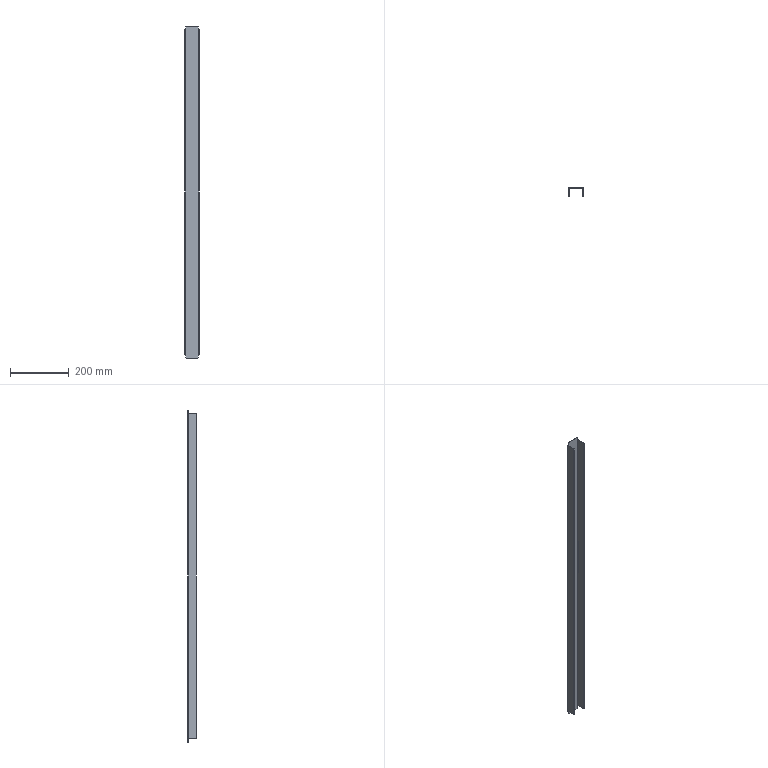Part | SolidWorks | features Chamfer 1, FlatPattern 1, ICE 1, SMBaseFlange 1, SheetMetal 1 | 1 solid | 26 faces | box 50 x 30 x 1127 mm | volume 233640 mm3 | plane 22 | cylinder 4 | commonest cylinder face diameters 0.4 x2 4.4 x2
STEP:
#1=CARTESIAN_POINT('',(-19.,-2.,563.5));
#2=VERTEX_POINT('',#1);
#3=CARTESIAN_POINT('',(19.,-2.,563.5));
#4=VERTEX_POINT('',#3);
#5=CARTESIAN_POINT('',(-25.,-2.,563.5));
#6=DIRECTION('',(1.,0.,0.));
#7=VECTOR('',#6,1000.);
#8=LINE('',#5,#7);
#9=EDGE_CURVE('',#2,#4,#8,.T.);
#10=ORIENTED_EDGE('',*,*,#9,.T.);
#11=CARTESIAN_POINT('',(19.,0.,563.5));
#12=VERTEX_POINT('',#11);
#13=CARTESIAN_POINT('',(19.,0.,563.5));
#14=DIRECTION('',(0.,1.,0.));
#15=VECTOR('',#14,1000.);
#16=LINE('',#13,#15);
#17=EDGE_CURVE('',#4,#12,#16,.T.);
#18=ORIENTED_EDGE('',*,*,#17,.T.);
#19=CARTESIAN_POINT('',(-19.,0.,563.5));
#20=VERTEX_POINT('',#19);
#21=CARTESIAN_POINT('',(-25.,0.,563.5));
#22=DIRECTION('',(1.,0.,0.));
#23=VECTOR('',#22,1000.);
#24=LINE('',#21,#23);
#25=EDGE_CURVE('',#20,#12,#24,.T.);
#26=ORIENTED_EDGE('',*,*,#25,.F.);
#27=CARTESIAN_POINT('',(-19.,-2.,563.5));
#28=DIRECTION('',(0.,-1.,0.));
#29=VECTOR('',#28,1000.);
#30=LINE('',#27,#29);
#31=EDGE_CURVE('',#20,#2,#30,.T.);
#32=ORIENTED_EDGE('',*,*,#31,.T.);
#33=EDGE_LOOP('',(#10,#18,#26,#32));
#34=FACE_OUTER_BOUND('',#33,.T.);
#35=CARTESIAN_POINT('',(-23.,-2.2,563.5));
#36=DIRECTION('',(0.,0.,1.));
#37=DIRECTION('',(1.,0.,0.));
#38=AXIS2_PLACEMENT_3D('',#35,#36,#37);
#39=PLANE('',#38);
#40=ADVANCED_FACE('',(#34),#39,.T.);
#41=CARTESIAN_POINT('',(-19.,0.,-563.5));
#42=VERTEX_POINT('',#41);
#43=CARTESIAN_POINT('',(19.,0.,-563.5));
#44=VERTEX_POINT('',#43);
#45=CARTESIAN_POINT('',(-25.,0.,-563.5));
#46=DIRECTION('',(1.,0.,0.));
#47=VECTOR('',#46,1000.);
#48=LINE('',#45,#47);
#49=EDGE_CURVE('',#42,#44,#48,.T.);
#50=ORIENTED_EDGE('',*,*,#49,.T.);
#51=CARTESIAN_POINT('',(19.,-2.,-563.5));
#52=VERTEX_POINT('',#51);
#53=CARTESIAN_POINT('',(19.,-2.,-563.5));
#54=DIRECTION('',(0.,-1.,0.));
#55=VECTOR('',#54,1000.);
#56=LINE('',#53,#55);
#57=EDGE_CURVE('',#44,#52,#56,.T.);
#58=ORIENTED_EDGE('',*,*,#57,.T.);
#59=CARTESIAN_POINT('',(-19.,-2.,-563.5));
#60=VERTEX_POINT('',#59);
#61=CARTESIAN_POINT('',(-25.,-2.,-563.5));
#62=DIRECTION('',(1.,0.,0.));
#63=VECTOR('',#62,1000.);
#64=LINE('',#61,#63);
#65=EDGE_CURVE('',#60,#52,#64,.T.);
#66=ORIENTED_EDGE('',*,*,#65,.F.);
#67=CARTESIAN_POINT('',(-19.,0.,-563.5));
#68=DIRECTION('',(0.,1.,0.));
#69=VECTOR('',#68,1000.);
#70=LINE('',#67,#69);
#71=EDGE_CURVE('',#60,#42,#70,.T.);
#72=ORIENTED_EDGE('',*,*,#71,.T.);
#73=EDGE_LOOP('',(#50,#58,#66,#72));
#74=FACE_OUTER_BOUND('',#73,.T.);
#75=CARTESIAN_POINT('',(23.,-2.2,-563.5));
#76=DIRECTION('',(0.,0.,-1.));
#77=DIRECTION('',(-1.,0.,0.));
#78=AXIS2_PLACEMENT_3D('',#75,#76,#77);
#79=PLANE('',#78);
#80=ADVANCED_FACE('',(#74),#79,.T.);
#81=CARTESIAN_POINT('',(23.,-2.2,551.5));
#82=VERTEX_POINT('',#81);
#83=CARTESIAN_POINT('',(23.,-2.2,-551.5));
#84=VERTEX_POINT('',#83);
#85=CARTESIAN_POINT('',(23.,-2.2,563.5));
#86=DIRECTION('',(0.,0.,-1.));
#87=VECTOR('',#86,1000.);
#88=LINE('',#85,#87);
#89=EDGE_CURVE('',#82,#84,#88,.T.);
#90=ORIENTED_EDGE('',*,*,#89,.T.);
#91=CARTESIAN_POINT('',(23.,-30.,-551.5));
#92=VERTEX_POINT('',#91);
#93=CARTESIAN_POINT('',(23.,0.,-551.5));
#94=DIRECTION('',(0.,-1.,0.));
#95=VECTOR('',#94,1000.);
#96=LINE('',#93,#95);
#97=EDGE_CURVE('',#84,#92,#96,.T.);
#98=ORIENTED_EDGE('',*,*,#97,.T.);
#99=CARTESIAN_POINT('',(23.,-30.,551.5));
#100=VERTEX_POINT('',#99);
#101=CARTESIAN_POINT('',(23.,-30.,563.5));
#102=DIRECTION('',(0.,0.,-1.));
#103=VECTOR('',#102,1000.);
#104=LINE('',#101,#103);
#105=EDGE_CURVE('',#100,#92,#104,.T.);
#106=ORIENTED_EDGE('',*,*,#105,.F.);
#107=CARTESIAN_POINT('',(23.,0.,551.5));
#108=DIRECTION('',(0.,1.,0.));
#109=VECTOR('',#108,1000.);
#110=LINE('',#107,#109);
#111=EDGE_CURVE('',#100,#82,#110,.T.);
#112=ORIENTED_EDGE('',*,*,#111,.T.);
#113=EDGE_LOOP('',(#90,#98,#106,#112));
#114=FACE_OUTER_BOUND('',#113,.T.);
#115=CARTESIAN_POINT('',(23.,0.,563.5));
#116=DIRECTION('',(1.,0.,0.));
#117=DIRECTION('',(0.,1.,0.));
#118=AXIS2_PLACEMENT_3D('',#115,#116,#117);
#119=PLANE('',#118);
#120=ADVANCED_FACE('',(#114),#119,.F.);
#121=CARTESIAN_POINT('',(25.,-30.,-551.5));
#122=VERTEX_POINT('',#121);
#123=CARTESIAN_POINT('',(25.,-30.,-551.5));
#124=DIRECTION('',(1.,0.,0.));
#125=VECTOR('',#124,1000.);
#126=LINE('',#123,#125);
#127=EDGE_CURVE('',#92,#122,#126,.T.);
#128=ORIENTED_EDGE('',*,*,#127,.T.);
#129=CARTESIAN_POINT('',(25.,-30.,551.5));
#130=VERTEX_POINT('',#129);
#131=CARTESIAN_POINT('',(25.,-30.,563.5));
#132=DIRECTION('',(0.,0.,-1.));
#133=VECTOR('',#132,1000.);
#134=LINE('',#131,#133);
#135=EDGE_CURVE('',#130,#122,#134,.T.);
#136=ORIENTED_EDGE('',*,*,#135,.F.);
#137=CARTESIAN_POINT('',(25.,-30.,551.5));
#138=DIRECTION('',(-1.,0.,0.));
#139=VECTOR('',#138,1000.);
#140=LINE('',#137,#139);
#141=EDGE_CURVE('',#130,#100,#140,.T.);
#142=ORIENTED_EDGE('',*,*,#141,.T.);
#143=ORIENTED_EDGE('',*,*,#105,.T.);
#144=EDGE_LOOP('',(#128,#136,#142,#143));
#145=FACE_OUTER_BOUND('',#144,.T.);
#146=CARTESIAN_POINT('',(25.,-30.,563.5));
#147=DIRECTION('',(0.,-1.,0.));
#148=DIRECTION('',(1.,0.,0.));
#149=AXIS2_PLACEMENT_3D('',#146,#147,#148);
#150=PLANE('',#149);
#151=ADVANCED_FACE('',(#145),#150,.T.);
#152=CARTESIAN_POINT('',(25.,-2.2,-551.5));
#153=VERTEX_POINT('',#152);
#154=CARTESIAN_POINT('',(25.,-30.,-551.5));
#155=DIRECTION('',(0.,1.,0.));
#156=VECTOR('',#155,1000.);
#157=LINE('',#154,#156);
#158=EDGE_CURVE('',#122,#153,#157,.T.);
#159=ORIENTED_EDGE('',*,*,#158,.T.);
#160=CARTESIAN_POINT('',(25.,-2.2,551.5));
#161=VERTEX_POINT('',#160);
#162=CARTESIAN_POINT('',(25.,-2.2,563.5));
#163=DIRECTION('',(0.,0.,-1.));
#164=VECTOR('',#163,1000.);
#165=LINE('',#162,#164);
#166=EDGE_CURVE('',#161,#153,#165,.T.);
#167=ORIENTED_EDGE('',*,*,#166,.F.);
#168=CARTESIAN_POINT('',(25.,-30.,551.5));
#169=DIRECTION('',(0.,1.,0.));
#170=VECTOR('',#169,1000.);
#171=LINE('',#168,#170);
#172=EDGE_CURVE('',#130,#161,#171,.T.);
#173=ORIENTED_EDGE('',*,*,#172,.F.);
#174=ORIENTED_EDGE('',*,*,#135,.T.);
#175=EDGE_LOOP('',(#159,#167,#173,#174));
#176=FACE_OUTER_BOUND('',#175,.T.);
#177=CARTESIAN_POINT('',(25.,0.,563.5));
#178=DIRECTION('',(1.,0.,0.));
#179=DIRECTION('',(0.,1.,0.));
#180=AXIS2_PLACEMENT_3D('',#177,#178,#179);
#181=PLANE('',#180);
#182=ADVANCED_FACE('',(#176),#181,.T.);
#183=CARTESIAN_POINT('',(22.8,0.,-551.5));
#184=VERTEX_POINT('',#183);
#185=CARTESIAN_POINT('',(22.8,-2.2,-551.5));
#186=DIRECTION('',(0.,0.,-1.));
#187=DIRECTION('',(1.,0.,0.));
#188=AXIS2_PLACEMENT_3D('',#185,#186,#187);
#189=CIRCLE('',#188,2.2);
#190=EDGE_CURVE('',#184,#153,#189,.T.);
#191=ORIENTED_EDGE('',*,*,#190,.F.);
#192=CARTESIAN_POINT('',(22.8,0.,551.5));
#193=VERTEX_POINT('',#192);
#194=CARTESIAN_POINT('',(22.8,0.,563.5));
#195=DIRECTION('',(0.,0.,-1.));
#196=VECTOR('',#195,1000.);
#197=LINE('',#194,#196);
#198=EDGE_CURVE('',#193,#184,#197,.T.);
#199=ORIENTED_EDGE('',*,*,#198,.F.);
#200=CARTESIAN_POINT('',(22.8,-2.2,551.5));
#201=DIRECTION('',(0.,0.,1.));
#202=DIRECTION('',(-1.,0.,0.));
#203=AXIS2_PLACEMENT_3D('',#200,#201,#202);
#204=CIRCLE('',#203,2.2);
#205=EDGE_CURVE('',#161,#193,#204,.T.);
#206=ORIENTED_EDGE('',*,*,#205,.F.);
#207=ORIENTED_EDGE('',*,*,#166,.T.);
#208=EDGE_LOOP('',(#191,#199,#206,#207));
#209=FACE_OUTER_BOUND('',#208,.T.);
#210=CARTESIAN_POINT('',(22.8,-2.2,563.5));
#211=DIRECTION('',(0.,0.,-1.));
#212=DIRECTION('',(-1.,0.,0.));
#213=AXIS2_PLACEMENT_3D('',#210,#211,#212);
#214=CYLINDRICAL_SURFACE('',#213,2.2);
#215=ADVANCED_FACE('',(#209),#214,.T.);
#216=CARTESIAN_POINT('',(22.,0.,-560.5));
#217=VERTEX_POINT('',#216);
#218=CARTESIAN_POINT('',(22.,0.,-551.5));
#219=VERTEX_POINT('',#218);
#220=CARTESIAN_POINT('',(22.,0.,563.5));
#221=DIRECTION('',(0.,0.,1.));
#222=VECTOR('',#221,1000.);
#223=LINE('',#220,#222);
#224=EDGE_CURVE('',#217,#219,#223,.T.);
#225=ORIENTED_EDGE('',*,*,#224,.F.);
#226=CARTESIAN_POINT('',(560.5,0.,-22.));
#227=DIRECTION('',(-0.7071,0.,-0.7071));
#228=VECTOR('',#227,1000.);
#229=LINE('',#226,#228);
#230=EDGE_CURVE('',#217,#44,#229,.T.);
#231=ORIENTED_EDGE('',*,*,#230,.T.);
#232=ORIENTED_EDGE('',*,*,#49,.F.);
#233=CARTESIAN_POINT('',(-22.,0.,-560.5));
#234=VERTEX_POINT('',#233);
#235=CARTESIAN_POINT('',(-585.5,0.,3.));
#236=DIRECTION('',(-0.7071,0.,0.7071));
#237=VECTOR('',#236,1000.);
#238=LINE('',#235,#237);
#239=EDGE_CURVE('',#42,#234,#238,.T.);
#240=ORIENTED_EDGE('',*,*,#239,.T.);
#241=CARTESIAN_POINT('',(-22.,0.,-551.5));
#242=VERTEX_POINT('',#241);
#243=CARTESIAN_POINT('',(-22.,0.,563.5));
#244=DIRECTION('',(0.,0.,-1.));
#245=VECTOR('',#244,1000.);
#246=LINE('',#243,#245);
#247=EDGE_CURVE('',#242,#234,#246,.T.);
#248=ORIENTED_EDGE('',*,*,#247,.F.);
#249=CARTESIAN_POINT('',(-22.8,0.,-551.5));
#250=VERTEX_POINT('',#249);
#251=CARTESIAN_POINT('',(-25.,0.,-551.5));
#252=DIRECTION('',(1.,0.,0.));
#253=VECTOR('',#252,1000.);
#254=LINE('',#251,#253);
#255=EDGE_CURVE('',#250,#242,#254,.T.);
#256=ORIENTED_EDGE('',*,*,#255,.F.);
#257=CARTESIAN_POINT('',(-22.8,0.,551.5));
#258=VERTEX_POINT('',#257);
#259=CARTESIAN_POINT('',(-22.8,0.,563.5));
#260=DIRECTION('',(0.,0.,-1.));
#261=VECTOR('',#260,1000.);
#262=LINE('',#259,#261);
#263=EDGE_CURVE('',#258,#250,#262,.T.);
#264=ORIENTED_EDGE('',*,*,#263,.F.);
#265=CARTESIAN_POINT('',(-22.,0.,551.5));
#266=VERTEX_POINT('',#265);
#267=CARTESIAN_POINT('',(-25.,0.,551.5));
#268=DIRECTION('',(-1.,0.,0.));
#269=VECTOR('',#268,1000.);
#270=LINE('',#267,#269);
#271=EDGE_CURVE('',#266,#258,#270,.T.);
#272=ORIENTED_EDGE('',*,*,#271,.F.);
#273=CARTESIAN_POINT('',(-22.,0.,560.5));
#274=VERTEX_POINT('',#273);
#275=CARTESIAN_POINT('',(-22.,0.,563.5));
#276=DIRECTION('',(0.,0.,-1.));
#277=VECTOR('',#276,1000.);
#278=LINE('',#275,#277);
#279=EDGE_CURVE('',#274,#266,#278,.T.);
#280=ORIENTED_EDGE('',*,*,#279,.F.);
#281=CARTESIAN_POINT('',(-22.,0.,560.5));
#282=DIRECTION('',(0.7071,0.,0.7071));
#283=VECTOR('',#282,1000.);
#284=LINE('',#281,#283);
#285=EDGE_CURVE('',#274,#20,#284,.T.);
#286=ORIENTED_EDGE('',*,*,#285,.T.);
#287=ORIENTED_EDGE('',*,*,#25,.T.);
#288=CARTESIAN_POINT('',(22.,0.,560.5));
#289=VERTEX_POINT('',#288);
#290=CARTESIAN_POINT('',(-3.,0.,585.5));
#291=DIRECTION('',(0.7071,0.,-0.7071));
#292=VECTOR('',#291,1000.);
#293=LINE('',#290,#292);
#294=EDGE_CURVE('',#12,#289,#293,.T.);
#295=ORIENTED_EDGE('',*,*,#294,.T.);
#296=CARTESIAN_POINT('',(22.,0.,551.5));
#297=VERTEX_POINT('',#296);
#298=CARTESIAN_POINT('',(22.,0.,563.5));
#299=DIRECTION('',(0.,0.,1.));
#300=VECTOR('',#299,1000.);
#301=LINE('',#298,#300);
#302=EDGE_CURVE('',#297,#289,#301,.T.);
#303=ORIENTED_EDGE('',*,*,#302,.F.);
#304=CARTESIAN_POINT('',(-25.,0.,551.5));
#305=DIRECTION('',(-1.,0.,0.));
#306=VECTOR('',#305,1000.);
#307=LINE('',#304,#306);
#308=EDGE_CURVE('',#193,#297,#307,.T.);
#309=ORIENTED_EDGE('',*,*,#308,.F.);
#310=ORIENTED_EDGE('',*,*,#198,.T.);
#311=CARTESIAN_POINT('',(-25.,0.,-551.5));
#312=DIRECTION('',(1.,0.,0.));
#313=VECTOR('',#312,1000.);
#314=LINE('',#311,#313);
#315=EDGE_CURVE('',#219,#184,#314,.T.);
#316=ORIENTED_EDGE('',*,*,#315,.F.);
#317=EDGE_LOOP('',(#225,#231,#232,#240,#248,#256,#264,#272,#280,#286,#287,#295,#303,#309,#310,#316));
#318=FACE_OUTER_BOUND('',#317,.T.);
#319=CARTESIAN_POINT('',(-25.,0.,563.5));
#320=DIRECTION('',(0.,1.,0.));
#321=DIRECTION('',(-1.,0.,0.));
#322=AXIS2_PLACEMENT_3D('',#319,#320,#321);
#323=PLANE('',#322);
#324=ADVANCED_FACE('',(#318),#323,.T.);
#325=CARTESIAN_POINT('',(-25.,-2.2,551.5));
#326=VERTEX_POINT('',#325);
#327=CARTESIAN_POINT('',(-22.8,-2.2,551.5));
#328=DIRECTION('',(0.,0.,1.));
#329=DIRECTION('',(-1.,0.,0.));
#330=AXIS2_PLACEMENT_3D('',#327,#328,#329);
#331=CIRCLE('',#330,2.2);
#332=EDGE_CURVE('',#258,#326,#331,.T.);
#333=ORIENTED_EDGE('',*,*,#332,.F.);
#334=ORIENTED_EDGE('',*,*,#263,.T.);
#335=CARTESIAN_POINT('',(-25.,-2.2,-551.5));
#336=VERTEX_POINT('',#335);
#337=CARTESIAN_POINT('',(-22.8,-2.2,-551.5));
#338=DIRECTION('',(0.,0.,-1.));
#339=DIRECTION('',(1.,0.,0.));
#340=AXIS2_PLACEMENT_3D('',#337,#338,#339);
#341=CIRCLE('',#340,2.2);
#342=EDGE_CURVE('',#336,#250,#341,.T.);
#343=ORIENTED_EDGE('',*,*,#342,.F.);
#344=CARTESIAN_POINT('',(-25.,-2.2,563.5));
#345=DIRECTION('',(0.,0.,-1.));
#346=VECTOR('',#345,1000.);
#347=LINE('',#344,#346);
#348=EDGE_CURVE('',#326,#336,#347,.T.);
#349=ORIENTED_EDGE('',*,*,#348,.F.);
#350=EDGE_LOOP('',(#333,#334,#343,#349));
#351=FACE_OUTER_BOUND('',#350,.T.);
#352=CARTESIAN_POINT('',(-22.8,-2.2,563.5));
#353=DIRECTION('',(0.,0.,-1.));
#354=DIRECTION('',(-1.,0.,0.));
#355=AXIS2_PLACEMENT_3D('',#352,#353,#354);
#356=CYLINDRICAL_SURFACE('',#355,2.2);
#357=ADVANCED_FACE('',(#351),#356,.T.);
#358=CARTESIAN_POINT('',(-25.,-30.,551.5));
#359=VERTEX_POINT('',#358);
#360=CARTESIAN_POINT('',(-25.,-30.,551.5));
#361=DIRECTION('',(0.,1.,0.));
#362=VECTOR('',#361,1000.);
#363=LINE('',#360,#362);
#364=EDGE_CURVE('',#359,#326,#363,.T.);
#365=ORIENTED_EDGE('',*,*,#364,.T.);
#366=ORIENTED_EDGE('',*,*,#348,.T.);
#367=CARTESIAN_POINT('',(-25.,-30.,-551.5));
#368=VERTEX_POINT('',#367);
#369=CARTESIAN_POINT('',(-25.,-30.,-551.5));
#370=DIRECTION('',(0.,1.,0.));
#371=VECTOR('',#370,1000.);
#372=LINE('',#369,#371);
#373=EDGE_CURVE('',#368,#336,#372,.T.);
#374=ORIENTED_EDGE('',*,*,#373,.F.);
#375=CARTESIAN_POINT('',(-25.,-30.,563.5));
#376=DIRECTION('',(0.,0.,-1.));
#377=VECTOR('',#376,1000.);
#378=LINE('',#375,#377);
#379=EDGE_CURVE('',#359,#368,#378,.T.);
#380=ORIENTED_EDGE('',*,*,#379,.F.);
#381=EDGE_LOOP('',(#365,#366,#374,#380));
#382=FACE_OUTER_BOUND('',#381,.T.);
#383=CARTESIAN_POINT('',(-25.,-30.,563.5));
#384=DIRECTION('',(-1.,0.,0.));
#385=DIRECTION('',(0.,0.,1.));
#386=AXIS2_PLACEMENT_3D('',#383,#384,#385);
#387=PLANE('',#386);
#388=ADVANCED_FACE('',(#382),#387,.T.);
#389=CARTESIAN_POINT('',(-23.,-30.,551.5));
#390=VERTEX_POINT('',#389);
#391=CARTESIAN_POINT('',(-25.,-30.,551.5));
#392=DIRECTION('',(-1.,0.,0.));
#393=VECTOR('',#392,1000.);
#394=LINE('',#391,#393);
#395=EDGE_CURVE('',#390,#359,#394,.T.);
#396=ORIENTED_EDGE('',*,*,#395,.T.);
#397=ORIENTED_EDGE('',*,*,#379,.T.);
#398=CARTESIAN_POINT('',(-23.,-30.,-551.5));
#399=VERTEX_POINT('',#398);
#400=CARTESIAN_POINT('',(-25.,-30.,-551.5));
#401=DIRECTION('',(1.,0.,0.));
#402=VECTOR('',#401,1000.);
#403=LINE('',#400,#402);
#404=EDGE_CURVE('',#368,#399,#403,.T.);
#405=ORIENTED_EDGE('',*,*,#404,.T.);
#406=CARTESIAN_POINT('',(-23.,-30.,563.5));
#407=DIRECTION('',(0.,0.,-1.));
#408=VECTOR('',#407,1000.);
#409=LINE('',#406,#408);
#410=EDGE_CURVE('',#390,#399,#409,.T.);
#411=ORIENTED_EDGE('',*,*,#410,.F.);
#412=EDGE_LOOP('',(#396,#397,#405,#411));
#413=FACE_OUTER_BOUND('',#412,.T.);
#414=CARTESIAN_POINT('',(-23.,-30.,563.5));
#415=DIRECTION('',(0.,-1.,0.));
#416=DIRECTION('',(0.,0.,-1.));
#417=AXIS2_PLACEMENT_3D('',#414,#415,#416);
#418=PLANE('',#417);
#419=ADVANCED_FACE('',(#413),#418,.T.);
#420=CARTESIAN_POINT('',(-23.,-2.2,551.5));
#421=VERTEX_POINT('',#420);
#422=CARTESIAN_POINT('',(-23.,-2.2,-551.5));
#423=VERTEX_POINT('',#422);
#424=CARTESIAN_POINT('',(-23.,-2.2,563.5));
#425=DIRECTION('',(0.,0.,-1.));
#426=VECTOR('',#425,1000.);
#427=LINE('',#424,#426);
#428=EDGE_CURVE('',#421,#423,#427,.T.);
#429=ORIENTED_EDGE('',*,*,#428,.F.);
#430=CARTESIAN_POINT('',(-23.,-30.,551.5));
#431=DIRECTION('',(0.,-1.,0.));
#432=VECTOR('',#431,1000.);
#433=LINE('',#430,#432);
#434=EDGE_CURVE('',#421,#390,#433,.T.);
#435=ORIENTED_EDGE('',*,*,#434,.T.);
#436=ORIENTED_EDGE('',*,*,#410,.T.);
#437=CARTESIAN_POINT('',(-23.,-30.,-551.5));
#438=DIRECTION('',(0.,1.,0.));
#439=VECTOR('',#438,1000.);
#440=LINE('',#437,#439);
#441=EDGE_CURVE('',#399,#423,#440,.T.);
#442=ORIENTED_EDGE('',*,*,#441,.T.);
#443=EDGE_LOOP('',(#429,#435,#436,#442));
#444=FACE_OUTER_BOUND('',#443,.T.);
#445=CARTESIAN_POINT('',(-23.,-30.,563.5));
#446=DIRECTION('',(-1.,0.,0.));
#447=DIRECTION('',(0.,0.,1.));
#448=AXIS2_PLACEMENT_3D('',#445,#446,#447);
#449=PLANE('',#448);
#450=ADVANCED_FACE('',(#444),#449,.F.);
#451=CARTESIAN_POINT('',(-22.8,-2.,551.5));
#452=VERTEX_POINT('',#451);
#453=CARTESIAN_POINT('',(-22.8,-2.,-551.5));
#454=VERTEX_POINT('',#453);
#455=CARTESIAN_POINT('',(-22.8,-2.,563.5));
#456=DIRECTION('',(0.,0.,-1.));
#457=VECTOR('',#456,1000.);
#458=LINE('',#455,#457);
#459=EDGE_CURVE('',#452,#454,#458,.T.);
#460=ORIENTED_EDGE('',*,*,#459,.F.);
#461=CARTESIAN_POINT('',(-22.8,-2.2,551.5));
#462=DIRECTION('',(0.,0.,1.));
#463=DIRECTION('',(-1.,0.,0.));
#464=AXIS2_PLACEMENT_3D('',#461,#462,#463);
#465=CIRCLE('',#464,0.2);
#466=EDGE_CURVE('',#452,#421,#465,.T.);
#467=ORIENTED_EDGE('',*,*,#466,.T.);
#468=ORIENTED_EDGE('',*,*,#428,.T.);
#469=CARTESIAN_POINT('',(-22.8,-2.2,-551.5));
#470=DIRECTION('',(0.,0.,-1.));
#471=DIRECTION('',(1.,0.,0.));
#472=AXIS2_PLACEMENT_3D('',#469,#470,#471);
#473=CIRCLE('',#472,0.2);
#474=EDGE_CURVE('',#423,#454,#473,.T.);
#475=ORIENTED_EDGE('',*,*,#474,.T.);
#476=EDGE_LOOP('',(#460,#467,#468,#475));
#477=FACE_OUTER_BOUND('',#476,.T.);
#478=CARTESIAN_POINT('',(-22.8,-2.2,563.5));
#479=DIRECTION('',(0.,0.,-1.));
#480=DIRECTION('',(-1.,0.,0.));
#481=AXIS2_PLACEMENT_3D('',#478,#479,#480);
#482=CYLINDRICAL_SURFACE('',#481,0.2);
#483=ADVANCED_FACE('',(#477),#482,.F.);
#484=ORIENTED_EDGE('',*,*,#65,.T.);
#485=CARTESIAN_POINT('',(22.,-2.,-560.5));
#486=VERTEX_POINT('',#485);
#487=CARTESIAN_POINT('',(22.,-2.,-560.5));
#488=DIRECTION('',(0.7071,0.,0.7071));
#489=VECTOR('',#488,1000.);
#490=LINE('',#487,#489);
#491=EDGE_CURVE('',#52,#486,#490,.T.);
#492=ORIENTED_EDGE('',*,*,#491,.T.);
#493=CARTESIAN_POINT('',(22.,-2.,-551.5));
#494=VERTEX_POINT('',#493);
#495=CARTESIAN_POINT('',(22.,-2.,563.5));
#496=DIRECTION('',(0.,0.,1.));
#497=VECTOR('',#496,1000.);
#498=LINE('',#495,#497);
#499=EDGE_CURVE('',#486,#494,#498,.T.);
#500=ORIENTED_EDGE('',*,*,#499,.T.);
#501=CARTESIAN_POINT('',(22.8,-2.,-551.5));
#502=VERTEX_POINT('',#501);
#503=CARTESIAN_POINT('',(-25.,-2.,-551.5));
#504=DIRECTION('',(1.,0.,0.));
#505=VECTOR('',#504,1000.);
#506=LINE('',#503,#505);
#507=EDGE_CURVE('',#494,#502,#506,.T.);
#508=ORIENTED_EDGE('',*,*,#507,.T.);
#509=CARTESIAN_POINT('',(22.8,-2.,551.5));
#510=VERTEX_POINT('',#509);
#511=CARTESIAN_POINT('',(22.8,-2.,563.5));
#512=DIRECTION('',(0.,0.,-1.));
#513=VECTOR('',#512,1000.);
#514=LINE('',#511,#513);
#515=EDGE_CURVE('',#510,#502,#514,.T.);
#516=ORIENTED_EDGE('',*,*,#515,.F.);
#517=CARTESIAN_POINT('',(22.,-2.,551.5));
#518=VERTEX_POINT('',#517);
#519=CARTESIAN_POINT('',(-25.,-2.,551.5));
#520=DIRECTION('',(-1.,0.,0.));
#521=VECTOR('',#520,1000.);
#522=LINE('',#519,#521);
#523=EDGE_CURVE('',#510,#518,#522,.T.);
#524=ORIENTED_EDGE('',*,*,#523,.T.);
#525=CARTESIAN_POINT('',(22.,-2.,560.5));
#526=VERTEX_POINT('',#525);
#527=CARTESIAN_POINT('',(22.,-2.,563.5));
#528=DIRECTION('',(0.,0.,1.));
#529=VECTOR('',#528,1000.);
#530=LINE('',#527,#529);
#531=EDGE_CURVE('',#518,#526,#530,.T.);
#532=ORIENTED_EDGE('',*,*,#531,.T.);
#533=CARTESIAN_POINT('',(19.,-2.,563.5));
#534=DIRECTION('',(-0.7071,0.,0.7071));
#535=VECTOR('',#534,1000.);
#536=LINE('',#533,#535);
#537=EDGE_CURVE('',#526,#4,#536,.T.);
#538=ORIENTED_EDGE('',*,*,#537,.T.);
#539=ORIENTED_EDGE('',*,*,#9,.F.);
#540=CARTESIAN_POINT('',(-22.,-2.,560.5));
#541=VERTEX_POINT('',#540);
#542=CARTESIAN_POINT('',(-22.,-2.,560.5));
#543=DIRECTION('',(-0.7071,0.,-0.7071));
#544=VECTOR('',#543,1000.);
#545=LINE('',#542,#544);
#546=EDGE_CURVE('',#2,#541,#545,.T.);
#547=ORIENTED_EDGE('',*,*,#546,.T.);
#548=CARTESIAN_POINT('',(-22.,-2.,551.5));
#549=VERTEX_POINT('',#548);
#550=CARTESIAN_POINT('',(-22.,-2.,563.5));
#551=DIRECTION('',(0.,0.,-1.));
#552=VECTOR('',#551,1000.);
#553=LINE('',#550,#552);
#554=EDGE_CURVE('',#541,#549,#553,.T.);
#555=ORIENTED_EDGE('',*,*,#554,.T.);
#556=CARTESIAN_POINT('',(-25.,-2.,551.5));
#557=DIRECTION('',(-1.,0.,0.));
#558=VECTOR('',#557,1000.);
#559=LINE('',#556,#558);
#560=EDGE_CURVE('',#549,#452,#559,.T.);
#561=ORIENTED_EDGE('',*,*,#560,.T.);
#562=ORIENTED_EDGE('',*,*,#459,.T.);
#563=CARTESIAN_POINT('',(-22.,-2.,-551.5));
#564=VERTEX_POINT('',#563);
#565=CARTESIAN_POINT('',(-25.,-2.,-551.5));
#566=DIRECTION('',(1.,0.,0.));
#567=VECTOR('',#566,1000.);
#568=LINE('',#565,#567);
#569=EDGE_CURVE('',#454,#564,#568,.T.);
#570=ORIENTED_EDGE('',*,*,#569,.T.);
#571=CARTESIAN_POINT('',(-22.,-2.,-560.5));
#572=VERTEX_POINT('',#571);
#573=CARTESIAN_POINT('',(-22.,-2.,563.5));
#574=DIRECTION('',(0.,0.,-1.));
#575=VECTOR('',#574,1000.);
#576=LINE('',#573,#575);
#577=EDGE_CURVE('',#564,#572,#576,.T.);
#578=ORIENTED_EDGE('',*,*,#577,.T.);
#579=CARTESIAN_POINT('',(-19.,-2.,-563.5));
#580=DIRECTION('',(0.7071,0.,-0.7071));
#581=VECTOR('',#580,1000.);
#582=LINE('',#579,#581);
#583=EDGE_CURVE('',#572,#60,#582,.T.);
#584=ORIENTED_EDGE('',*,*,#583,.T.);
#585=EDGE_LOOP('',(#484,#492,#500,#508,#516,#524,#532,#538,#539,#547,#555,#561,#562,#570,#578,#584));
#586=FACE_OUTER_BOUND('',#585,.T.);
#587=CARTESIAN_POINT('',(-25.,-2.,563.5));
#588=DIRECTION('',(0.,1.,0.));
#589=DIRECTION('',(-1.,0.,0.));
#590=AXIS2_PLACEMENT_3D('',#587,#588,#589);
#591=PLANE('',#590);
#592=ADVANCED_FACE('',(#586),#591,.F.);
#593=ORIENTED_EDGE('',*,*,#515,.T.);
#594=CARTESIAN_POINT('',(22.8,-2.2,-551.5));
#595=DIRECTION('',(0.,0.,-1.));
#596=DIRECTION('',(1.,0.,0.));
#597=AXIS2_PLACEMENT_3D('',#594,#595,#596);
#598=CIRCLE('',#597,0.2);
#599=EDGE_CURVE('',#502,#84,#598,.T.);
#600=ORIENTED_EDGE('',*,*,#599,.T.);
#601=ORIENTED_EDGE('',*,*,#89,.F.);
#602=CARTESIAN_POINT('',(22.8,-2.2,551.5));
#603=DIRECTION('',(0.,0.,1.));
#604=DIRECTION('',(-1.,0.,0.));
#605=AXIS2_PLACEMENT_3D('',#602,#603,#604);
#606=CIRCLE('',#605,0.2);
#607=EDGE_CURVE('',#82,#510,#606,.T.);
#608=ORIENTED_EDGE('',*,*,#607,.T.);
#609=EDGE_LOOP('',(#593,#600,#601,#608));
#610=FACE_OUTER_BOUND('',#609,.T.);
#611=CARTESIAN_POINT('',(22.8,-2.2,563.5));
#612=DIRECTION('',(0.,0.,-1.));
#613=DIRECTION('',(-1.,0.,0.));
#614=AXIS2_PLACEMENT_3D('',#611,#612,#613);
#615=CYLINDRICAL_SURFACE('',#614,0.2);
#616=ADVANCED_FACE('',(#610),#615,.F.);
#617=ORIENTED_EDGE('',*,*,#302,.T.);
#618=CARTESIAN_POINT('',(22.,-2.,560.5));
#619=DIRECTION('',(0.,-1.,0.));
#620=VECTOR('',#619,1000.);
#621=LINE('',#618,#620);
#622=EDGE_CURVE('',#289,#526,#621,.T.);
#623=ORIENTED_EDGE('',*,*,#622,.T.);
#624=ORIENTED_EDGE('',*,*,#531,.F.);
#625=CARTESIAN_POINT('',(22.,-30.,551.5));
#626=DIRECTION('',(0.,1.,0.));
#627=VECTOR('',#626,1000.);
#628=LINE('',#625,#627);
#629=EDGE_CURVE('',#518,#297,#628,.T.);
#630=ORIENTED_EDGE('',*,*,#629,.T.);
#631=EDGE_LOOP('',(#617,#623,#624,#630));
#632=FACE_OUTER_BOUND('',#631,.T.);
#633=CARTESIAN_POINT('',(22.,-30.,563.5));
#634=DIRECTION('',(-1.,0.,0.));
#635=DIRECTION('',(0.,0.,1.));
#636=AXIS2_PLACEMENT_3D('',#633,#634,#635);
#637=PLANE('',#636);
#638=ADVANCED_FACE('',(#632),#637,.F.);
#639=ORIENTED_EDGE('',*,*,#205,.T.);
#640=ORIENTED_EDGE('',*,*,#308,.T.);
#641=ORIENTED_EDGE('',*,*,#629,.F.);
#642=ORIENTED_EDGE('',*,*,#523,.F.);
#643=ORIENTED_EDGE('',*,*,#607,.F.);
#644=ORIENTED_EDGE('',*,*,#111,.F.);
#645=ORIENTED_EDGE('',*,*,#141,.F.);
#646=ORIENTED_EDGE('',*,*,#172,.T.);
#647=EDGE_LOOP('',(#639,#640,#641,#642,#643,#644,#645,#646));
#648=FACE_OUTER_BOUND('',#647,.T.);
#649=CARTESIAN_POINT('',(25.,-30.,551.5));
#650=DIRECTION('',(0.,0.,-1.));
#651=DIRECTION('',(-1.,0.,0.));
#652=AXIS2_PLACEMENT_3D('',#649,#650,#651);
#653=PLANE('',#652);
#654=ADVANCED_FACE('',(#648),#653,.F.);
#655=ORIENTED_EDGE('',*,*,#499,.F.);
#656=CARTESIAN_POINT('',(22.,0.,-560.5));
#657=DIRECTION('',(0.,1.,0.));
#658=VECTOR('',#657,1000.);
#659=LINE('',#656,#658);
#660=EDGE_CURVE('',#486,#217,#659,.T.);
#661=ORIENTED_EDGE('',*,*,#660,.T.);
#662=ORIENTED_EDGE('',*,*,#224,.T.);
#663=CARTESIAN_POINT('',(22.,-30.,-551.5));
#664=DIRECTION('',(0.,1.,0.));
#665=VECTOR('',#664,1000.);
#666=LINE('',#663,#665);
#667=EDGE_CURVE('',#494,#219,#666,.T.);
#668=ORIENTED_EDGE('',*,*,#667,.F.);
#669=EDGE_LOOP('',(#655,#661,#662,#668));
#670=FACE_OUTER_BOUND('',#669,.T.);
#671=CARTESIAN_POINT('',(22.,-30.,-563.5));
#672=DIRECTION('',(-1.,0.,0.));
#673=DIRECTION('',(0.,0.,1.));
#674=AXIS2_PLACEMENT_3D('',#671,#672,#673);
#675=PLANE('',#674);
#676=ADVANCED_FACE('',(#670),#675,.F.);
#677=ORIENTED_EDGE('',*,*,#190,.T.);
#678=ORIENTED_EDGE('',*,*,#158,.F.);
#679=ORIENTED_EDGE('',*,*,#127,.F.);
#680=ORIENTED_EDGE('',*,*,#97,.F.);
#681=ORIENTED_EDGE('',*,*,#599,.F.);
#682=ORIENTED_EDGE('',*,*,#507,.F.);
#683=ORIENTED_EDGE('',*,*,#667,.T.);
#684=ORIENTED_EDGE('',*,*,#315,.T.);
#685=EDGE_LOOP('',(#677,#678,#679,#680,#681,#682,#683,#684));
#686=FACE_OUTER_BOUND('',#685,.T.);
#687=CARTESIAN_POINT('',(25.,-30.,-551.5));
#688=DIRECTION('',(0.,0.,1.));
#689=DIRECTION('',(1.,0.,0.));
#690=AXIS2_PLACEMENT_3D('',#687,#688,#689);
#691=PLANE('',#690);
#692=ADVANCED_FACE('',(#686),#691,.F.);
#693=ORIENTED_EDGE('',*,*,#247,.T.);
#694=CARTESIAN_POINT('',(-22.,-2.,-560.5));
#695=DIRECTION('',(0.,-1.,0.));
#696=VECTOR('',#695,1000.);
#697=LINE('',#694,#696);
#698=EDGE_CURVE('',#234,#572,#697,.T.);
#699=ORIENTED_EDGE('',*,*,#698,.T.);
#700=ORIENTED_EDGE('',*,*,#577,.F.);
#701=CARTESIAN_POINT('',(-22.,-30.,-551.5));
#702=DIRECTION('',(0.,1.,0.));
#703=VECTOR('',#702,1000.);
#704=LINE('',#701,#703);
#705=EDGE_CURVE('',#564,#242,#704,.T.);
#706=ORIENTED_EDGE('',*,*,#705,.T.);
#707=EDGE_LOOP('',(#693,#699,#700,#706));
#708=FACE_OUTER_BOUND('',#707,.T.);
#709=CARTESIAN_POINT('',(-22.,-30.,-563.5));
#710=DIRECTION('',(1.,0.,0.));
#711=DIRECTION('',(0.,0.,-1.));
#712=AXIS2_PLACEMENT_3D('',#709,#710,#711);
#713=PLANE('',#712);
#714=ADVANCED_FACE('',(#708),#713,.F.);
#715=ORIENTED_EDGE('',*,*,#255,.T.);
#716=ORIENTED_EDGE('',*,*,#705,.F.);
#717=ORIENTED_EDGE('',*,*,#569,.F.);
#718=ORIENTED_EDGE('',*,*,#474,.F.);
#719=ORIENTED_EDGE('',*,*,#441,.F.);
#720=ORIENTED_EDGE('',*,*,#404,.F.);
#721=ORIENTED_EDGE('',*,*,#373,.T.);
#722=ORIENTED_EDGE('',*,*,#342,.T.);
#723=EDGE_LOOP('',(#715,#716,#717,#718,#719,#720,#721,#722));
#724=FACE_OUTER_BOUND('',#723,.T.);
#725=CARTESIAN_POINT('',(-25.,-30.,-551.5));
#726=DIRECTION('',(0.,0.,1.));
#727=DIRECTION('',(1.,0.,0.));
#728=AXIS2_PLACEMENT_3D('',#725,#726,#727);
#729=PLANE('',#728);
#730=ADVANCED_FACE('',(#724),#729,.F.);
#731=ORIENTED_EDGE('',*,*,#271,.T.);
#732=ORIENTED_EDGE('',*,*,#332,.T.);
#733=ORIENTED_EDGE('',*,*,#364,.F.);
#734=ORIENTED_EDGE('',*,*,#395,.F.);
#735=ORIENTED_EDGE('',*,*,#434,.F.);
#736=ORIENTED_EDGE('',*,*,#466,.F.);
#737=ORIENTED_EDGE('',*,*,#560,.F.);
#738=CARTESIAN_POINT('',(-22.,-30.,551.5));
#739=DIRECTION('',(0.,1.,0.));
#740=VECTOR('',#739,1000.);
#741=LINE('',#738,#740);
#742=EDGE_CURVE('',#549,#266,#741,.T.);
#743=ORIENTED_EDGE('',*,*,#742,.T.);
#744=EDGE_LOOP('',(#731,#732,#733,#734,#735,#736,#737,#743));
#745=FACE_OUTER_BOUND('',#744,.T.);
#746=CARTESIAN_POINT('',(-25.,-30.,551.5));
#747=DIRECTION('',(0.,0.,-1.));
#748=DIRECTION('',(-1.,0.,0.));
#749=AXIS2_PLACEMENT_3D('',#746,#747,#748);
#750=PLANE('',#749);
#751=ADVANCED_FACE('',(#745),#750,.F.);
#752=ORIENTED_EDGE('',*,*,#554,.F.);
#753=CARTESIAN_POINT('',(-22.,0.,560.5));
#754=DIRECTION('',(0.,1.,0.));
#755=VECTOR('',#754,1000.);
#756=LINE('',#753,#755);
#757=EDGE_CURVE('',#541,#274,#756,.T.);
#758=ORIENTED_EDGE('',*,*,#757,.T.);
#759=ORIENTED_EDGE('',*,*,#279,.T.);
#760=ORIENTED_EDGE('',*,*,#742,.F.);
#761=EDGE_LOOP('',(#752,#758,#759,#760));
#762=FACE_OUTER_BOUND('',#761,.T.);
#763=CARTESIAN_POINT('',(-22.,-30.,563.5));
#764=DIRECTION('',(1.,0.,0.));
#765=DIRECTION('',(0.,0.,-1.));
#766=AXIS2_PLACEMENT_3D('',#763,#764,#765);
#767=PLANE('',#766);
#768=ADVANCED_FACE('',(#762),#767,.F.);
#769=ORIENTED_EDGE('',*,*,#491,.F.);
#770=ORIENTED_EDGE('',*,*,#57,.F.);
#771=ORIENTED_EDGE('',*,*,#230,.F.);
#772=ORIENTED_EDGE('',*,*,#660,.F.);
#773=EDGE_LOOP('',(#769,#770,#771,#772));
#774=FACE_OUTER_BOUND('',#773,.T.);
#775=CARTESIAN_POINT('',(22.,-30.,-560.5));
#776=DIRECTION('',(0.7071,0.,-0.7071));
#777=DIRECTION('',(0.,-1.,0.));
#778=AXIS2_PLACEMENT_3D('',#775,#776,#777);
#779=PLANE('',#778);
#780=ADVANCED_FACE('',(#774),#779,.T.);
#781=ORIENTED_EDGE('',*,*,#583,.F.);
#782=ORIENTED_EDGE('',*,*,#698,.F.);
#783=ORIENTED_EDGE('',*,*,#239,.F.);
#784=ORIENTED_EDGE('',*,*,#71,.F.);
#785=EDGE_LOOP('',(#781,#782,#783,#784));
#786=FACE_OUTER_BOUND('',#785,.T.);
#787=CARTESIAN_POINT('',(-19.,-2.2,-563.5));
#788=DIRECTION('',(-0.7071,0.,-0.7071));
#789=DIRECTION('',(0.,-1.,0.));
#790=AXIS2_PLACEMENT_3D('',#787,#788,#789);
#791=PLANE('',#790);
#792=ADVANCED_FACE('',(#786),#791,.T.);
#793=ORIENTED_EDGE('',*,*,#537,.F.);
#794=ORIENTED_EDGE('',*,*,#622,.F.);
#795=ORIENTED_EDGE('',*,*,#294,.F.);
#796=ORIENTED_EDGE('',*,*,#17,.F.);
#797=EDGE_LOOP('',(#793,#794,#795,#796));
#798=FACE_OUTER_BOUND('',#797,.T.);
#799=CARTESIAN_POINT('',(19.,-2.2,563.5));
#800=DIRECTION('',(0.7071,0.,0.7071));
#801=DIRECTION('',(0.,-1.,0.));
#802=AXIS2_PLACEMENT_3D('',#799,#800,#801);
#803=PLANE('',#802);
#804=ADVANCED_FACE('',(#798),#803,.T.);
#805=ORIENTED_EDGE('',*,*,#546,.F.);
#806=ORIENTED_EDGE('',*,*,#31,.F.);
#807=ORIENTED_EDGE('',*,*,#285,.F.);
#808=ORIENTED_EDGE('',*,*,#757,.F.);
#809=EDGE_LOOP('',(#805,#806,#807,#808));
#810=FACE_OUTER_BOUND('',#809,.T.);
#811=CARTESIAN_POINT('',(-22.,-30.,560.5));
#812=DIRECTION('',(-0.7071,0.,0.7071));
#813=DIRECTION('',(0.,-1.,0.));
#814=AXIS2_PLACEMENT_3D('',#811,#812,#813);
#815=PLANE('',#814);
#816=ADVANCED_FACE('',(#810),#815,.T.);
#817=CLOSED_SHELL('',(#40,#80,#120,#151,#182,#215,#324,#357,#388,#419,#450,#483,#592,#616,#638,#654,#676,#692,#714,#730,#751,#768,#780,#792,#804,#816));
#818=MANIFOLD_SOLID_BREP('',#817);
#819=CARTESIAN_POINT('',(0.,0.,0.));
#820=DIRECTION('',(0.,0.,1.));
#821=DIRECTION('',(1.,0.,0.));
#822=AXIS2_PLACEMENT_3D('',#819,#820,#821);
#823=(LENGTH_UNIT()NAMED_UNIT(*)SI_UNIT(.MILLI.,.METRE.));
#824=UNCERTAINTY_MEASURE_WITH_UNIT(LENGTH_MEASURE(0.00001),#823,'','');
#825=(NAMED_UNIT(*)PLANE_ANGLE_UNIT()SI_UNIT($,.RADIAN.));
#826=(NAMED_UNIT(*)SI_UNIT($,.STERADIAN.)SOLID_ANGLE_UNIT());
#827=(GEOMETRIC_REPRESENTATION_CONTEXT(3)GLOBAL_UNCERTAINTY_ASSIGNED_CONTEXT((#824))GLOBAL_UNIT_ASSIGNED_CONTEXT((#823,#825,#826))REPRESENTATION_CONTEXT('',''));
#828=ADVANCED_BREP_SHAPE_REPRESENTATION('',(#818,#822),#827);